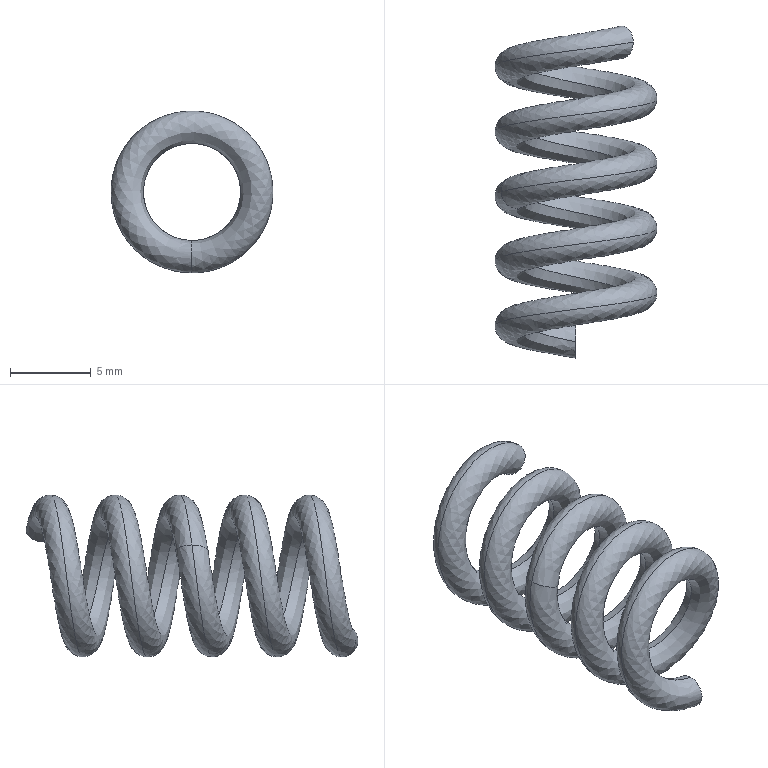Part | NX | features solid 2 | 1 solid | 6 faces | box 10 x 20.499 x 10 mm | volume 364.957 mm3 | spline 4 | plane 2